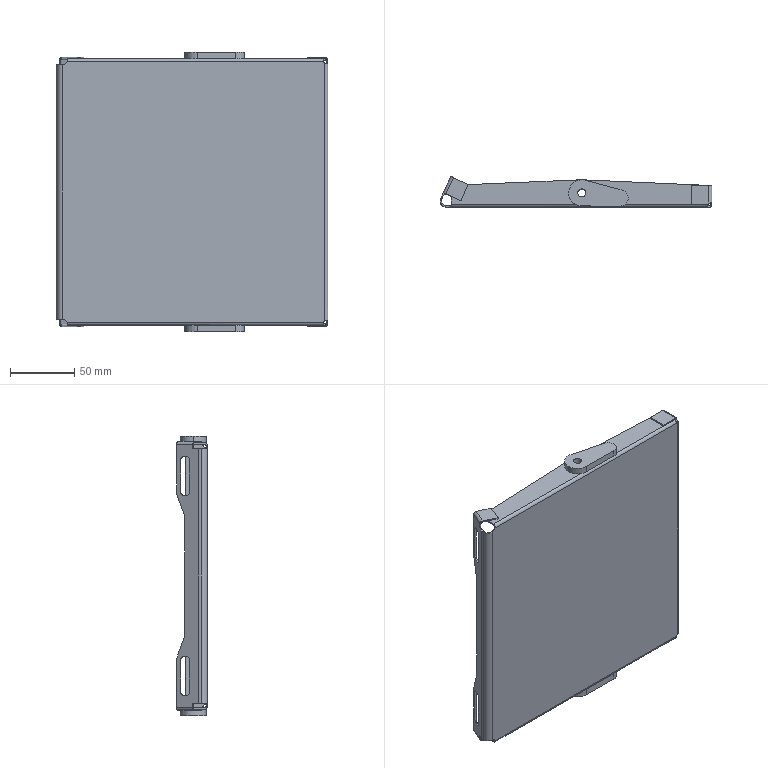Part | SolidWorks | features BaseBody 3 | 3 solids | 118 faces | box 210.716 x 23.81 x 216.939 mm | volume 65530 mm3 | plane 58 | cylinder 52 | spline 8 | commonest cylinder face diameters 5.08 x8 5.678 x8 6.35 x8 2.54 x7 4.572 x7 20.32 x5